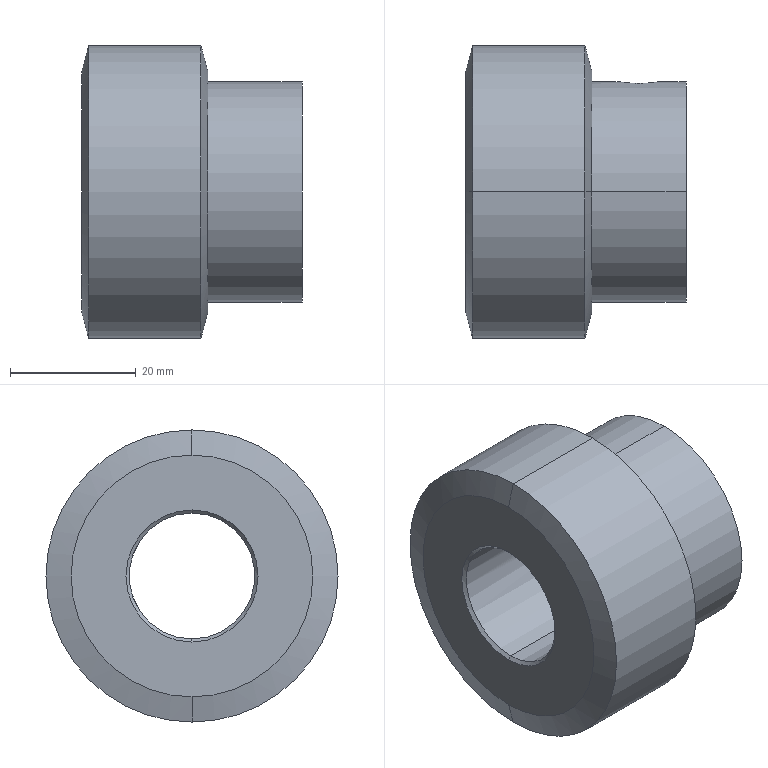Part | SolidWorks | features BaseBody 1 | 1 solid | 26 faces | box 35 x 46.43 x 46.43 mm | volume 36544 mm3 | cone 12 | cylinder 11 | plane 3 | commonest cylinder face diameters 6 x3 4.917 x2 20 x2 35 x2 46.43 x2
STEP:
#1=CARTESIAN_POINT('',(27.5,10.542,-2.459));
#2=VERTEX_POINT('',#1);
#3=CARTESIAN_POINT('',(27.5,10.542,2.459));
#4=VERTEX_POINT('',#3);
#5=CARTESIAN_POINT('',(27.5,10.542,0.));
#6=DIRECTION('',(0.,1.,0.));
#7=DIRECTION('',(0.,0.,1.));
#8=AXIS2_PLACEMENT_3D('',#5,#6,#7);
#9=CIRCLE('',#8,2.459);
#10=EDGE_CURVE('',#2,#4,#9,.T.);
#11=ORIENTED_EDGE('',*,*,#10,.T.);
#12=CARTESIAN_POINT('',(27.5,10.,3.));
#13=VERTEX_POINT('',#12);
#14=CARTESIAN_POINT('',(27.5,10.,3.));
#15=DIRECTION('',(0.,-0.7071,0.7071));
#16=VECTOR('',#15,1000.);
#17=LINE('',#14,#16);
#18=EDGE_CURVE('',#4,#13,#17,.T.);
#19=ORIENTED_EDGE('',*,*,#18,.T.);
#20=CARTESIAN_POINT('',(24.5,10.,0.));
#21=VERTEX_POINT('',#20);
#22=CARTESIAN_POINT('',(27.5,10.,0.));
#23=DIRECTION('',(0.,1.,0.));
#24=DIRECTION('',(0.,0.,1.));
#25=AXIS2_PLACEMENT_3D('',#22,#23,#24);
#26=CIRCLE('',#25,3.);
#27=EDGE_CURVE('',#21,#13,#26,.T.);
#28=ORIENTED_EDGE('',*,*,#27,.F.);
#29=CARTESIAN_POINT('',(27.5,10.,-3.));
#30=VERTEX_POINT('',#29);
#31=CARTESIAN_POINT('',(27.5,10.,0.));
#32=DIRECTION('',(0.,1.,0.));
#33=DIRECTION('',(0.,0.,1.));
#34=AXIS2_PLACEMENT_3D('',#31,#32,#33);
#35=CIRCLE('',#34,3.);
#36=EDGE_CURVE('',#30,#21,#35,.T.);
#37=ORIENTED_EDGE('',*,*,#36,.F.);
#38=CARTESIAN_POINT('',(27.5,10.,-3.));
#39=DIRECTION('',(0.,-0.7071,-0.7071));
#40=VECTOR('',#39,1000.);
#41=LINE('',#38,#40);
#42=EDGE_CURVE('',#2,#30,#41,.T.);
#43=ORIENTED_EDGE('',*,*,#42,.F.);
#44=EDGE_LOOP('',(#11,#19,#28,#37,#43));
#45=FACE_OUTER_BOUND('',#44,.T.);
#46=CARTESIAN_POINT('',(27.5,10.,0.));
#47=DIRECTION('',(0.,-1.,0.));
#48=DIRECTION('',(0.,0.,-1.));
#49=AXIS2_PLACEMENT_3D('',#46,#47,#48);
#50=CONICAL_SURFACE('',#49,3.,0.7854);
#51=ADVANCED_FACE('',(#45),#50,.F.);
#52=ORIENTED_EDGE('',*,*,#10,.F.);
#53=CARTESIAN_POINT('',(27.5,16.959,-2.459));
#54=VERTEX_POINT('',#53);
#55=CARTESIAN_POINT('',(27.5,0.,-2.459));
#56=DIRECTION('',(0.,1.,0.));
#57=VECTOR('',#56,1000.);
#58=LINE('',#55,#57);
#59=EDGE_CURVE('',#2,#54,#58,.T.);
#60=ORIENTED_EDGE('',*,*,#59,.T.);
#61=CARTESIAN_POINT('',(27.5,16.959,2.459));
#62=VERTEX_POINT('',#61);
#63=CARTESIAN_POINT('',(27.5,16.959,0.));
#64=DIRECTION('',(0.,1.,0.));
#65=DIRECTION('',(0.,0.,1.));
#66=AXIS2_PLACEMENT_3D('',#63,#64,#65);
#67=CIRCLE('',#66,2.459);
#68=EDGE_CURVE('',#54,#62,#67,.T.);
#69=ORIENTED_EDGE('',*,*,#68,.T.);
#70=CARTESIAN_POINT('',(27.5,0.,2.459));
#71=DIRECTION('',(0.,1.,0.));
#72=VECTOR('',#71,1000.);
#73=LINE('',#70,#72);
#74=EDGE_CURVE('',#4,#62,#73,.T.);
#75=ORIENTED_EDGE('',*,*,#74,.F.);
#76=EDGE_LOOP('',(#52,#60,#69,#75));
#77=FACE_OUTER_BOUND('',#76,.T.);
#78=CARTESIAN_POINT('',(27.5,0.,0.));
#79=DIRECTION('',(0.,1.,0.));
#80=DIRECTION('',(0.,0.,1.));
#81=AXIS2_PLACEMENT_3D('',#78,#79,#80);
#82=CYLINDRICAL_SURFACE('',#81,2.459);
#83=ADVANCED_FACE('',(#77),#82,.F.);
#84=ORIENTED_EDGE('',*,*,#68,.F.);
#85=CARTESIAN_POINT('',(27.5,17.278,-2.778));
#86=VERTEX_POINT('',#85);
#87=CARTESIAN_POINT('',(27.5,16.959,-2.459));
#88=DIRECTION('',(0.,0.7071,-0.7071));
#89=VECTOR('',#88,1000.);
#90=LINE('',#87,#89);
#91=EDGE_CURVE('',#54,#86,#90,.T.);
#92=ORIENTED_EDGE('',*,*,#91,.T.);
#93=CARTESIAN_POINT('',(27.5,17.278,2.778));
#94=VERTEX_POINT('',#93);
#95=CARTESIAN_POINT('',(27.5,17.278,-2.778));
#96=CARTESIAN_POINT('',(27.309,17.278,-2.778));
#97=CARTESIAN_POINT('',(27.121,17.281,-2.761));
#98=CARTESIAN_POINT('',(26.751,17.291,-2.695));
#99=CARTESIAN_POINT('',(26.567,17.299,-2.646));
#100=CARTESIAN_POINT('',(26.211,17.319,-2.514));
#101=CARTESIAN_POINT('',(26.041,17.33,-2.433));
#102=CARTESIAN_POINT('',(25.718,17.356,-2.24));
#103=CARTESIAN_POINT('',(25.564,17.371,-2.128));
#104=CARTESIAN_POINT('',(25.281,17.4,-1.876));
#105=CARTESIAN_POINT('',(25.154,17.414,-1.739));
#106=CARTESIAN_POINT('',(24.928,17.441,-1.439));
#107=CARTESIAN_POINT('',(24.828,17.454,-1.274));
#108=CARTESIAN_POINT('',(24.668,17.476,-0.9326));
#109=CARTESIAN_POINT('',(24.606,17.485,-0.755));
#110=CARTESIAN_POINT('',(24.522,17.497,-0.3858));
#111=CARTESIAN_POINT('',(24.5,17.5,-0.1944));
#112=CARTESIAN_POINT('',(24.5,17.5,0.1826));
#113=CARTESIAN_POINT('',(24.52,17.497,0.3724));
#114=CARTESIAN_POINT('',(24.603,17.485,0.7441));
#115=CARTESIAN_POINT('',(24.664,17.477,0.9226));
#116=CARTESIAN_POINT('',(24.823,17.455,1.266));
#117=CARTESIAN_POINT('',(24.922,17.442,1.43));
#118=CARTESIAN_POINT('',(25.148,17.415,1.732));
#119=CARTESIAN_POINT('',(25.277,17.4,1.872));
#120=CARTESIAN_POINT('',(25.56,17.371,2.125));
#121=CARTESIAN_POINT('',(25.712,17.357,2.236));
#122=CARTESIAN_POINT('',(26.036,17.331,2.43));
#123=CARTESIAN_POINT('',(26.209,17.319,2.513));
#124=CARTESIAN_POINT('',(26.563,17.299,2.645));
#125=CARTESIAN_POINT('',(26.745,17.291,2.694));
#126=CARTESIAN_POINT('',(27.118,17.281,2.761));
#127=CARTESIAN_POINT('',(27.309,17.278,2.778));
#128=CARTESIAN_POINT('',(27.5,17.278,2.778));
#129=B_SPLINE_CURVE_WITH_KNOTS('',3,(#95,#96,#97,#98,#99,#100,#101,#102,#103,#104,#105,#106,#107,#108,#109,#110,#111,#112,#113,#114,#115,#116,#117,#118,#119,#120,#121,#122,#123,#124,#125,#126,#127,#128),.UNSPECIFIED.,.F.,.F.,(4,2,2,2,2,2,2,2,2,2,2,2,2,2,2,2,4),(0.,0.0005647,0.001129,0.001694,0.002259,0.002823,0.003388,0.003953,0.004517,0.005082,0.005647,0.006211,0.006776,0.007341,0.007905,0.00847,0.009035),.UNSPECIFIED.);
#130=EDGE_CURVE('',#86,#94,#129,.T.);
#131=ORIENTED_EDGE('',*,*,#130,.T.);
#132=CARTESIAN_POINT('',(27.5,16.959,2.459));
#133=DIRECTION('',(0.,0.7071,0.7071));
#134=VECTOR('',#133,1000.);
#135=LINE('',#132,#134);
#136=EDGE_CURVE('',#62,#94,#135,.T.);
#137=ORIENTED_EDGE('',*,*,#136,.F.);
#138=EDGE_LOOP('',(#84,#92,#131,#137));
#139=FACE_OUTER_BOUND('',#138,.T.);
#140=CARTESIAN_POINT('',(27.5,16.959,0.));
#141=DIRECTION('',(0.,1.,0.));
#142=DIRECTION('',(0.,0.,1.));
#143=AXIS2_PLACEMENT_3D('',#140,#141,#142);
#144=CONICAL_SURFACE('',#143,2.459,0.7854);
#145=ADVANCED_FACE('',(#139),#144,.F.);
#146=CARTESIAN_POINT('',(30.5,10.,0.));
#147=VERTEX_POINT('',#146);
#148=CARTESIAN_POINT('',(27.5,9.539,3.));
#149=VERTEX_POINT('',#148);
#150=CARTESIAN_POINT('',(30.5,10.,0.));
#151=CARTESIAN_POINT('',(30.5,10.,0.1993));
#152=CARTESIAN_POINT('',(30.48,9.994,0.3951));
#153=CARTESIAN_POINT('',(30.403,9.971,0.7799));
#154=CARTESIAN_POINT('',(30.345,9.954,0.971));
#155=CARTESIAN_POINT('',(30.194,9.912,1.334));
#156=CARTESIAN_POINT('',(30.102,9.887,1.505));
#157=CARTESIAN_POINT('',(29.885,9.832,1.831));
#158=CARTESIAN_POINT('',(29.759,9.802,1.984));
#159=CARTESIAN_POINT('',(29.347,9.713,2.396));
#160=CARTESIAN_POINT('',(29.014,9.652,2.619));
#161=CARTESIAN_POINT('',(28.474,9.587,2.844));
#162=CARTESIAN_POINT('',(28.284,9.57,2.902));
#163=CARTESIAN_POINT('',(27.896,9.546,2.98));
#164=CARTESIAN_POINT('',(27.699,9.539,3.));
#165=CARTESIAN_POINT('',(27.5,9.539,3.));
#166=B_SPLINE_CURVE_WITH_KNOTS('',3,(#150,#151,#152,#153,#154,#155,#156,#157,#158,#159,#160,#161,#162,#163,#164,#165),.UNSPECIFIED.,.F.,.F.,(4,2,2,2,2,2,2,4),(0.,0.0005892,0.001178,0.001768,0.002357,0.003535,0.004125,0.004714),.UNSPECIFIED.);
#167=EDGE_CURVE('',#147,#149,#166,.T.);
#168=ORIENTED_EDGE('',*,*,#167,.T.);
#169=CARTESIAN_POINT('',(27.5,0.,3.));
#170=DIRECTION('',(0.,1.,0.));
#171=VECTOR('',#170,1000.);
#172=LINE('',#169,#171);
#173=EDGE_CURVE('',#149,#13,#172,.T.);
#174=ORIENTED_EDGE('',*,*,#173,.T.);
#175=CARTESIAN_POINT('',(27.5,10.,0.));
#176=DIRECTION('',(0.,1.,0.));
#177=DIRECTION('',(0.,0.,1.));
#178=AXIS2_PLACEMENT_3D('',#175,#176,#177);
#179=CIRCLE('',#178,3.);
#180=EDGE_CURVE('',#13,#147,#179,.T.);
#181=ORIENTED_EDGE('',*,*,#180,.T.);
#182=EDGE_LOOP('',(#168,#174,#181));
#183=FACE_OUTER_BOUND('',#182,.T.);
#184=CARTESIAN_POINT('',(27.5,0.,0.));
#185=DIRECTION('',(0.,1.,0.));
#186=DIRECTION('',(0.,0.,1.));
#187=AXIS2_PLACEMENT_3D('',#184,#185,#186);
#188=CYLINDRICAL_SURFACE('',#187,3.);
#189=ADVANCED_FACE('',(#183),#188,.F.);
#190=CARTESIAN_POINT('',(18.928,0.,23.215));
#191=VERTEX_POINT('',#190);
#192=CARTESIAN_POINT('',(18.928,0.,-23.215));
#193=VERTEX_POINT('',#192);
#194=CARTESIAN_POINT('',(18.928,0.,0.));
#195=DIRECTION('',(-1.,0.,0.));
#196=DIRECTION('',(0.,0.,1.));
#197=AXIS2_PLACEMENT_3D('',#194,#195,#196);
#198=CIRCLE('',#197,23.215);
#199=EDGE_CURVE('',#191,#193,#198,.T.);
#200=ORIENTED_EDGE('',*,*,#199,.T.);
#201=CARTESIAN_POINT('',(1.072,0.,-23.215));
#202=VERTEX_POINT('',#201);
#203=CARTESIAN_POINT('',(35.,0.,-23.215));
#204=DIRECTION('',(-1.,0.,0.));
#205=VECTOR('',#204,1000.);
#206=LINE('',#203,#205);
#207=EDGE_CURVE('',#193,#202,#206,.T.);
#208=ORIENTED_EDGE('',*,*,#207,.T.);
#209=CARTESIAN_POINT('',(1.072,0.,23.215));
#210=VERTEX_POINT('',#209);
#211=CARTESIAN_POINT('',(1.072,0.,0.));
#212=DIRECTION('',(-1.,0.,0.));
#213=DIRECTION('',(0.,0.,1.));
#214=AXIS2_PLACEMENT_3D('',#211,#212,#213);
#215=CIRCLE('',#214,23.215);
#216=EDGE_CURVE('',#210,#202,#215,.T.);
#217=ORIENTED_EDGE('',*,*,#216,.F.);
#218=CARTESIAN_POINT('',(35.,0.,23.215));
#219=DIRECTION('',(-1.,0.,0.));
#220=VECTOR('',#219,1000.);
#221=LINE('',#218,#220);
#222=EDGE_CURVE('',#191,#210,#221,.T.);
#223=ORIENTED_EDGE('',*,*,#222,.F.);
#224=EDGE_LOOP('',(#200,#208,#217,#223));
#225=FACE_OUTER_BOUND('',#224,.T.);
#226=CARTESIAN_POINT('',(35.,0.,0.));
#227=DIRECTION('',(-1.,0.,0.));
#228=DIRECTION('',(0.,0.,1.));
#229=AXIS2_PLACEMENT_3D('',#226,#227,#228);
#230=CYLINDRICAL_SURFACE('',#229,23.215);
#231=ADVANCED_FACE('',(#225),#230,.T.);
#232=CARTESIAN_POINT('',(20.,0.,19.215));
#233=VERTEX_POINT('',#232);
#234=CARTESIAN_POINT('',(20.,0.,-19.215));
#235=VERTEX_POINT('',#234);
#236=CARTESIAN_POINT('',(20.,0.,0.));
#237=DIRECTION('',(-1.,0.,0.));
#238=DIRECTION('',(0.,0.,1.));
#239=AXIS2_PLACEMENT_3D('',#236,#237,#238);
#240=CIRCLE('',#239,19.215);
#241=EDGE_CURVE('',#233,#235,#240,.T.);
#242=ORIENTED_EDGE('',*,*,#241,.T.);
#243=CARTESIAN_POINT('',(20.,0.,-19.215));
#244=DIRECTION('',(-0.2588,0.,-0.9659));
#245=VECTOR('',#244,1000.);
#246=LINE('',#243,#245);
#247=EDGE_CURVE('',#235,#193,#246,.T.);
#248=ORIENTED_EDGE('',*,*,#247,.T.);
#249=ORIENTED_EDGE('',*,*,#199,.F.);
#250=CARTESIAN_POINT('',(20.,0.,19.215));
#251=DIRECTION('',(-0.2588,0.,0.9659));
#252=VECTOR('',#251,1000.);
#253=LINE('',#250,#252);
#254=EDGE_CURVE('',#233,#191,#253,.T.);
#255=ORIENTED_EDGE('',*,*,#254,.F.);
#256=EDGE_LOOP('',(#242,#248,#249,#255));
#257=FACE_OUTER_BOUND('',#256,.T.);
#258=CARTESIAN_POINT('',(20.,0.,0.));
#259=DIRECTION('',(-1.,0.,0.));
#260=DIRECTION('',(0.,0.,1.));
#261=AXIS2_PLACEMENT_3D('',#258,#259,#260);
#262=CONICAL_SURFACE('',#261,19.215,1.309);
#263=ADVANCED_FACE('',(#257),#262,.T.);
#264=CARTESIAN_POINT('',(34.5,0.,-10.));
#265=VERTEX_POINT('',#264);
#266=CARTESIAN_POINT('',(34.5,0.,10.));
#267=VERTEX_POINT('',#266);
#268=CARTESIAN_POINT('',(34.5,0.,0.));
#269=DIRECTION('',(-1.,0.,0.));
#270=DIRECTION('',(0.,0.,1.));
#271=AXIS2_PLACEMENT_3D('',#268,#269,#270);
#272=CIRCLE('',#271,10.);
#273=EDGE_CURVE('',#265,#267,#272,.T.);
#274=ORIENTED_EDGE('',*,*,#273,.T.);
#275=CARTESIAN_POINT('',(35.,0.,10.5));
#276=VERTEX_POINT('',#275);
#277=CARTESIAN_POINT('',(34.5,0.,10.));
#278=DIRECTION('',(0.7071,0.,0.7071));
#279=VECTOR('',#278,1000.);
#280=LINE('',#277,#279);
#281=EDGE_CURVE('',#267,#276,#280,.T.);
#282=ORIENTED_EDGE('',*,*,#281,.T.);
#283=CARTESIAN_POINT('',(35.,0.,-10.5));
#284=VERTEX_POINT('',#283);
#285=CARTESIAN_POINT('',(35.,0.,0.));
#286=DIRECTION('',(-1.,0.,0.));
#287=DIRECTION('',(0.,0.,1.));
#288=AXIS2_PLACEMENT_3D('',#285,#286,#287);
#289=CIRCLE('',#288,10.5);
#290=EDGE_CURVE('',#284,#276,#289,.T.);
#291=ORIENTED_EDGE('',*,*,#290,.F.);
#292=CARTESIAN_POINT('',(34.5,0.,-10.));
#293=DIRECTION('',(0.7071,0.,-0.7071));
#294=VECTOR('',#293,1000.);
#295=LINE('',#292,#294);
#296=EDGE_CURVE('',#265,#284,#295,.T.);
#297=ORIENTED_EDGE('',*,*,#296,.F.);
#298=EDGE_LOOP('',(#274,#282,#291,#297));
#299=FACE_OUTER_BOUND('',#298,.T.);
#300=CARTESIAN_POINT('',(34.5,0.,0.));
#301=DIRECTION('',(1.,0.,0.));
#302=DIRECTION('',(0.,0.,-1.));
#303=AXIS2_PLACEMENT_3D('',#300,#301,#302);
#304=CONICAL_SURFACE('',#303,10.,0.7854);
#305=ADVANCED_FACE('',(#299),#304,.F.);
#306=CARTESIAN_POINT('',(0.5,0.,-10.));
#307=VERTEX_POINT('',#306);
#308=CARTESIAN_POINT('',(0.5,0.,10.));
#309=VERTEX_POINT('',#308);
#310=CARTESIAN_POINT('',(0.5,0.,0.));
#311=DIRECTION('',(-1.,0.,0.));
#312=DIRECTION('',(0.,0.,1.));
#313=AXIS2_PLACEMENT_3D('',#310,#311,#312);
#314=CIRCLE('',#313,10.);
#315=EDGE_CURVE('',#307,#309,#314,.T.);
#316=ORIENTED_EDGE('',*,*,#315,.F.);
#317=CARTESIAN_POINT('',(0.,0.,-10.5));
#318=VERTEX_POINT('',#317);
#319=CARTESIAN_POINT('',(0.,0.,-10.5));
#320=DIRECTION('',(-0.7071,0.,-0.7071));
#321=VECTOR('',#320,1000.);
#322=LINE('',#319,#321);
#323=EDGE_CURVE('',#307,#318,#322,.T.);
#324=ORIENTED_EDGE('',*,*,#323,.T.);
#325=CARTESIAN_POINT('',(0.,0.,10.5));
#326=VERTEX_POINT('',#325);
#327=CARTESIAN_POINT('',(0.,0.,0.));
#328=DIRECTION('',(-1.,0.,0.));
#329=DIRECTION('',(0.,0.,1.));
#330=AXIS2_PLACEMENT_3D('',#327,#328,#329);
#331=CIRCLE('',#330,10.5);
#332=EDGE_CURVE('',#318,#326,#331,.T.);
#333=ORIENTED_EDGE('',*,*,#332,.T.);
#334=CARTESIAN_POINT('',(0.,0.,10.5));
#335=DIRECTION('',(-0.7071,0.,0.7071));
#336=VECTOR('',#335,1000.);
#337=LINE('',#334,#336);
#338=EDGE_CURVE('',#309,#326,#337,.T.);
#339=ORIENTED_EDGE('',*,*,#338,.F.);
#340=EDGE_LOOP('',(#316,#324,#333,#339));
#341=FACE_OUTER_BOUND('',#340,.T.);
#342=CARTESIAN_POINT('',(0.,0.,0.));
#343=DIRECTION('',(-1.,0.,0.));
#344=DIRECTION('',(0.,0.,1.));
#345=AXIS2_PLACEMENT_3D('',#342,#343,#344);
#346=CONICAL_SURFACE('',#345,10.5,0.7854);
#347=ADVANCED_FACE('',(#341),#346,.F.);
#348=CARTESIAN_POINT('',(0.,0.,19.215));
#349=VERTEX_POINT('',#348);
#350=CARTESIAN_POINT('',(0.,0.,-19.215));
#351=VERTEX_POINT('',#350);
#352=CARTESIAN_POINT('',(0.,0.,0.));
#353=DIRECTION('',(-1.,0.,0.));
#354=DIRECTION('',(0.,0.,1.));
#355=AXIS2_PLACEMENT_3D('',#352,#353,#354);
#356=CIRCLE('',#355,19.215);
#357=EDGE_CURVE('',#349,#351,#356,.T.);
#358=ORIENTED_EDGE('',*,*,#357,.F.);
#359=CARTESIAN_POINT('',(1.072,0.,23.215));
#360=DIRECTION('',(0.2588,0.,0.9659));
#361=VECTOR('',#360,1000.);
#362=LINE('',#359,#361);
#363=EDGE_CURVE('',#349,#210,#362,.T.);
#364=ORIENTED_EDGE('',*,*,#363,.T.);
#365=ORIENTED_EDGE('',*,*,#216,.T.);
#366=CARTESIAN_POINT('',(1.072,0.,-23.215));
#367=DIRECTION('',(0.2588,0.,-0.9659));
#368=VECTOR('',#367,1000.);
#369=LINE('',#366,#368);
#370=EDGE_CURVE('',#351,#202,#369,.T.);
#371=ORIENTED_EDGE('',*,*,#370,.F.);
#372=EDGE_LOOP('',(#358,#364,#365,#371));
#373=FACE_OUTER_BOUND('',#372,.T.);
#374=CARTESIAN_POINT('',(1.072,0.,0.));
#375=DIRECTION('',(1.,0.,0.));
#376=DIRECTION('',(0.,0.,-1.));
#377=AXIS2_PLACEMENT_3D('',#374,#375,#376);
#378=CONICAL_SURFACE('',#377,23.215,1.309);
#379=ADVANCED_FACE('',(#373),#378,.T.);
#380=CARTESIAN_POINT('',(27.5,17.278,2.778));
#381=CARTESIAN_POINT('',(27.691,17.278,2.778));
#382=CARTESIAN_POINT('',(27.879,17.281,2.761));
#383=CARTESIAN_POINT('',(28.249,17.291,2.695));
#384=CARTESIAN_POINT('',(28.433,17.299,2.646));
#385=CARTESIAN_POINT('',(28.789,17.319,2.514));
#386=CARTESIAN_POINT('',(28.959,17.33,2.433));
#387=CARTESIAN_POINT('',(29.282,17.356,2.24));
#388=CARTESIAN_POINT('',(29.436,17.371,2.128));
#389=CARTESIAN_POINT('',(29.719,17.4,1.876));
#390=CARTESIAN_POINT('',(29.846,17.414,1.739));
#391=CARTESIAN_POINT('',(30.072,17.441,1.439));
#392=CARTESIAN_POINT('',(30.172,17.454,1.274));
#393=CARTESIAN_POINT('',(30.332,17.476,0.9326));
#394=CARTESIAN_POINT('',(30.394,17.485,0.755));
#395=CARTESIAN_POINT('',(30.478,17.497,0.3858));
#396=CARTESIAN_POINT('',(30.5,17.5,0.1944));
#397=CARTESIAN_POINT('',(30.5,17.5,-0.1826));
#398=CARTESIAN_POINT('',(30.48,17.497,-0.3724));
#399=CARTESIAN_POINT('',(30.397,17.485,-0.7441));
#400=CARTESIAN_POINT('',(30.336,17.477,-0.9226));
#401=CARTESIAN_POINT('',(30.177,17.455,-1.266));
#402=CARTESIAN_POINT('',(30.078,17.442,-1.43));
#403=CARTESIAN_POINT('',(29.852,17.415,-1.732));
#404=CARTESIAN_POINT('',(29.723,17.4,-1.872));
#405=CARTESIAN_POINT('',(29.44,17.371,-2.125));
#406=CARTESIAN_POINT('',(29.288,17.357,-2.236));
#407=CARTESIAN_POINT('',(28.964,17.331,-2.43));
#408=CARTESIAN_POINT('',(28.791,17.319,-2.513));
#409=CARTESIAN_POINT('',(28.437,17.299,-2.645));
#410=CARTESIAN_POINT('',(28.255,17.291,-2.694));
#411=CARTESIAN_POINT('',(27.882,17.281,-2.761));
#412=CARTESIAN_POINT('',(27.691,17.278,-2.778));
#413=CARTESIAN_POINT('',(27.5,17.278,-2.778));
#414=B_SPLINE_CURVE_WITH_KNOTS('',3,(#380,#381,#382,#383,#384,#385,#386,#387,#388,#389,#390,#391,#392,#393,#394,#395,#396,#397,#398,#399,#400,#401,#402,#403,#404,#405,#406,#407,#408,#409,#410,#411,#412,#413),.UNSPECIFIED.,.F.,.F.,(4,2,2,2,2,2,2,2,2,2,2,2,2,2,2,2,4),(0.009035,0.009599,0.01016,0.01073,0.01129,0.01186,0.01242,0.01299,0.01355,0.01411,0.01468,0.01524,0.01581,0.01637,0.01694,0.0175,0.01806),.UNSPECIFIED.);
#415=EDGE_CURVE('',#94,#86,#414,.T.);
#416=ORIENTED_EDGE('',*,*,#415,.F.);
#417=ORIENTED_EDGE('',*,*,#130,.F.);
#418=EDGE_LOOP('',(#416,#417));
#419=FACE_BOUND('',#418,.T.);
#420=CARTESIAN_POINT('',(35.,0.,17.5));
#421=VERTEX_POINT('',#420);
#422=CARTESIAN_POINT('',(35.,0.,-17.5));
#423=VERTEX_POINT('',#422);
#424=CARTESIAN_POINT('',(35.,0.,0.));
#425=DIRECTION('',(-1.,0.,0.));
#426=DIRECTION('',(0.,0.,1.));
#427=AXIS2_PLACEMENT_3D('',#424,#425,#426);
#428=CIRCLE('',#427,17.5);
#429=EDGE_CURVE('',#421,#423,#428,.T.);
#430=ORIENTED_EDGE('',*,*,#429,.T.);
#431=CARTESIAN_POINT('',(20.,0.,-17.5));
#432=VERTEX_POINT('',#431);
#433=CARTESIAN_POINT('',(35.,0.,-17.5));
#434=DIRECTION('',(-1.,0.,0.));
#435=VECTOR('',#434,1000.);
#436=LINE('',#433,#435);
#437=EDGE_CURVE('',#423,#432,#436,.T.);
#438=ORIENTED_EDGE('',*,*,#437,.T.);
#439=CARTESIAN_POINT('',(20.,0.,17.5));
#440=VERTEX_POINT('',#439);
#441=CARTESIAN_POINT('',(20.,0.,0.));
#442=DIRECTION('',(-1.,0.,0.));
#443=DIRECTION('',(0.,0.,1.));
#444=AXIS2_PLACEMENT_3D('',#441,#442,#443);
#445=CIRCLE('',#444,17.5);
#446=EDGE_CURVE('',#440,#432,#445,.T.);
#447=ORIENTED_EDGE('',*,*,#446,.F.);
#448=CARTESIAN_POINT('',(35.,0.,17.5));
#449=DIRECTION('',(-1.,0.,0.));
#450=VECTOR('',#449,1000.);
#451=LINE('',#448,#450);
#452=EDGE_CURVE('',#421,#440,#451,.T.);
#453=ORIENTED_EDGE('',*,*,#452,.F.);
#454=EDGE_LOOP('',(#430,#438,#447,#453));
#455=FACE_OUTER_BOUND('',#454,.T.);
#456=CARTESIAN_POINT('',(35.,0.,0.));
#457=DIRECTION('',(-1.,0.,0.));
#458=DIRECTION('',(0.,0.,1.));
#459=AXIS2_PLACEMENT_3D('',#456,#457,#458);
#460=CYLINDRICAL_SURFACE('',#459,17.5);
#461=ADVANCED_FACE('',(#419,#455),#460,.T.);
#462=ORIENTED_EDGE('',*,*,#273,.F.);
#463=CARTESIAN_POINT('',(35.,0.,-10.));
#464=DIRECTION('',(-1.,0.,0.));
#465=VECTOR('',#464,1000.);
#466=LINE('',#463,#465);
#467=EDGE_CURVE('',#265,#307,#466,.T.);
#468=ORIENTED_EDGE('',*,*,#467,.T.);
#469=ORIENTED_EDGE('',*,*,#315,.T.);
#470=CARTESIAN_POINT('',(35.,0.,10.));
#471=DIRECTION('',(-1.,0.,0.));
#472=VECTOR('',#471,1000.);
#473=LINE('',#470,#472);
#474=EDGE_CURVE('',#267,#309,#473,.T.);
#475=ORIENTED_EDGE('',*,*,#474,.F.);
#476=EDGE_LOOP('',(#462,#468,#469,#475));
#477=FACE_OUTER_BOUND('',#476,.T.);
#478=CARTESIAN_POINT('',(35.,0.,0.));
#479=DIRECTION('',(-1.,0.,0.));
#480=DIRECTION('',(0.,0.,1.));
#481=AXIS2_PLACEMENT_3D('',#478,#479,#480);
#482=CYLINDRICAL_SURFACE('',#481,10.);
#483=ADVANCED_FACE('',(#477),#482,.F.);
#484=CARTESIAN_POINT('',(24.5,10.,0.));
#485=CARTESIAN_POINT('',(24.5,10.,-0.1994));
#486=CARTESIAN_POINT('',(24.52,9.994,-0.3952));
#487=CARTESIAN_POINT('',(24.597,9.971,-0.7801));
#488=CARTESIAN_POINT('',(24.655,9.954,-0.9713));
#489=CARTESIAN_POINT('',(24.806,9.912,-1.334));
#490=CARTESIAN_POINT('',(24.898,9.887,-1.506));
#491=CARTESIAN_POINT('',(25.116,9.832,-1.831));
#492=CARTESIAN_POINT('',(25.241,9.802,-1.984));
#493=CARTESIAN_POINT('',(25.654,9.713,-2.396));
#494=CARTESIAN_POINT('',(25.986,9.652,-2.619));
#495=CARTESIAN_POINT('',(26.527,9.587,-2.844));
#496=CARTESIAN_POINT('',(26.717,9.57,-2.903));
#497=CARTESIAN_POINT('',(27.105,9.546,-2.98));
#498=CARTESIAN_POINT('',(27.3,9.539,-3.));
#499=CARTESIAN_POINT('',(27.694,9.539,-3.));
#500=CARTESIAN_POINT('',(27.894,9.546,-2.981));
#501=CARTESIAN_POINT('',(28.28,9.569,-2.904));
#502=CARTESIAN_POINT('',(28.467,9.587,-2.847));
#503=CARTESIAN_POINT('',(28.832,9.63,-2.695));
#504=CARTESIAN_POINT('',(29.005,9.656,-2.602));
#505=CARTESIAN_POINT('',(29.329,9.712,-2.386));
#506=CARTESIAN_POINT('',(29.482,9.742,-2.261));
#507=CARTESIAN_POINT('',(29.759,9.802,-1.984));
#508=CARTESIAN_POINT('',(29.882,9.832,-1.834));
#509=CARTESIAN_POINT('',(30.1,9.887,-1.51));
#510=CARTESIAN_POINT('',(30.194,9.912,-1.334));
#511=CARTESIAN_POINT('',(30.345,9.954,-0.9731));
#512=CARTESIAN_POINT('',(30.402,9.971,-0.786));
#513=CARTESIAN_POINT('',(30.48,9.994,-0.3988));
#514=CARTESIAN_POINT('',(30.5,10.,-0.1994));
#515=CARTESIAN_POINT('',(30.5,10.,0.));
#516=B_SPLINE_CURVE_WITH_KNOTS('',3,(#484,#485,#486,#487,#488,#489,#490,#491,#492,#493,#494,#495,#496,#497,#498,#499,#500,#501,#502,#503,#504,#505,#506,#507,#508,#509,#510,#511,#512,#513,#514,#515),.UNSPECIFIED.,.F.,.F.,(4,2,2,2,2,2,2,2,2,2,2,2,2,2,2,4),(0.,0.0005894,0.001179,0.001768,0.002358,0.003537,0.004126,0.004715,0.005305,0.005894,0.006484,0.007073,0.007662,0.008252,0.008841,0.009431),.UNSPECIFIED.);
#517=EDGE_CURVE('',#21,#147,#516,.T.);
#518=ORIENTED_EDGE('',*,*,#517,.T.);
#519=CARTESIAN_POINT('',(27.5,10.,0.));
#520=DIRECTION('',(0.,1.,0.));
#521=DIRECTION('',(0.,0.,1.));
#522=AXIS2_PLACEMENT_3D('',#519,#520,#521);
#523=CIRCLE('',#522,3.);
#524=EDGE_CURVE('',#147,#30,#523,.T.);
#525=ORIENTED_EDGE('',*,*,#524,.T.);
#526=ORIENTED_EDGE('',*,*,#36,.T.);
#527=EDGE_LOOP('',(#518,#525,#526));
#528=FACE_OUTER_BOUND('',#527,.T.);
#529=CARTESIAN_POINT('',(27.5,0.,0.));
#530=DIRECTION('',(0.,1.,0.));
#531=DIRECTION('',(0.,0.,1.));
#532=AXIS2_PLACEMENT_3D('',#529,#530,#531);
#533=CYLINDRICAL_SURFACE('',#532,3.);
#534=ADVANCED_FACE('',(#528),#533,.F.);
#535=ORIENTED_EDGE('',*,*,#446,.T.);
#536=CARTESIAN_POINT('',(20.,0.,0.));
#537=DIRECTION('',(-1.,0.,0.));
#538=DIRECTION('',(0.,0.,1.));
#539=AXIS2_PLACEMENT_3D('',#536,#537,#538);
#540=CIRCLE('',#539,17.5);
#541=EDGE_CURVE('',#432,#440,#540,.T.);
#542=ORIENTED_EDGE('',*,*,#541,.T.);
#543=EDGE_LOOP('',(#535,#542));
#544=FACE_BOUND('',#543,.T.);
#545=ORIENTED_EDGE('',*,*,#241,.F.);
#546=CARTESIAN_POINT('',(20.,0.,0.));
#547=DIRECTION('',(-1.,0.,0.));
#548=DIRECTION('',(0.,0.,1.));
#549=AXIS2_PLACEMENT_3D('',#546,#547,#548);
#550=CIRCLE('',#549,19.215);
#551=EDGE_CURVE('',#235,#233,#550,.T.);
#552=ORIENTED_EDGE('',*,*,#551,.F.);
#553=EDGE_LOOP('',(#545,#552));
#554=FACE_OUTER_BOUND('',#553,.T.);
#555=CARTESIAN_POINT('',(20.,17.5,0.));
#556=DIRECTION('',(-1.,0.,0.));
#557=DIRECTION('',(0.,0.,1.));
#558=AXIS2_PLACEMENT_3D('',#555,#556,#557);
#559=PLANE('',#558);
#560=ADVANCED_FACE('',(#544,#554),#559,.F.);
#561=ORIENTED_EDGE('',*,*,#290,.T.);
#562=CARTESIAN_POINT('',(35.,0.,0.));
#563=DIRECTION('',(-1.,0.,0.));
#564=DIRECTION('',(0.,0.,1.));
#565=AXIS2_PLACEMENT_3D('',#562,#563,#564);
#566=CIRCLE('',#565,10.5);
#567=EDGE_CURVE('',#276,#284,#566,.T.);
#568=ORIENTED_EDGE('',*,*,#567,.T.);
#569=EDGE_LOOP('',(#561,#568));
#570=FACE_BOUND('',#569,.T.);
#571=ORIENTED_EDGE('',*,*,#429,.F.);
#572=CARTESIAN_POINT('',(35.,0.,0.));
#573=DIRECTION('',(-1.,0.,0.));
#574=DIRECTION('',(0.,0.,1.));
#575=AXIS2_PLACEMENT_3D('',#572,#573,#574);
#576=CIRCLE('',#575,17.5);
#577=EDGE_CURVE('',#423,#421,#576,.T.);
#578=ORIENTED_EDGE('',*,*,#577,.F.);
#579=EDGE_LOOP('',(#571,#578));
#580=FACE_OUTER_BOUND('',#579,.T.);
#581=CARTESIAN_POINT('',(35.,10.5,0.));
#582=DIRECTION('',(-1.,0.,0.));
#583=DIRECTION('',(0.,0.,1.));
#584=AXIS2_PLACEMENT_3D('',#581,#582,#583);
#585=PLANE('',#584);
#586=ADVANCED_FACE('',(#570,#580),#585,.F.);
#587=CARTESIAN_POINT('',(0.,0.,0.));
#588=DIRECTION('',(-1.,0.,0.));
#589=DIRECTION('',(0.,0.,1.));
#590=AXIS2_PLACEMENT_3D('',#587,#588,#589);
#591=CIRCLE('',#590,10.5);
#592=EDGE_CURVE('',#326,#318,#591,.T.);
#593=ORIENTED_EDGE('',*,*,#592,.F.);
#594=ORIENTED_EDGE('',*,*,#332,.F.);
#595=EDGE_LOOP('',(#593,#594));
#596=FACE_BOUND('',#595,.T.);
#597=CARTESIAN_POINT('',(0.,0.,0.));
#598=DIRECTION('',(-1.,0.,0.));
#599=DIRECTION('',(0.,0.,1.));
#600=AXIS2_PLACEMENT_3D('',#597,#598,#599);
#601=CIRCLE('',#600,19.215);
#602=EDGE_CURVE('',#351,#349,#601,.T.);
#603=ORIENTED_EDGE('',*,*,#602,.T.);
#604=ORIENTED_EDGE('',*,*,#357,.T.);
#605=EDGE_LOOP('',(#603,#604));
#606=FACE_OUTER_BOUND('',#605,.T.);
#607=CARTESIAN_POINT('',(0.,19.215,0.));
#608=DIRECTION('',(1.,0.,0.));
#609=DIRECTION('',(0.,1.,0.));
#610=AXIS2_PLACEMENT_3D('',#607,#608,#609);
#611=PLANE('',#610);
#612=ADVANCED_FACE('',(#596,#606),#611,.F.);
#613=ORIENTED_EDGE('',*,*,#467,.F.);
#614=CARTESIAN_POINT('',(34.5,0.,0.));
#615=DIRECTION('',(-1.,0.,0.));
#616=DIRECTION('',(0.,0.,1.));
#617=AXIS2_PLACEMENT_3D('',#614,#615,#616);
#618=CIRCLE('',#617,10.);
#619=EDGE_CURVE('',#267,#265,#618,.T.);
#620=ORIENTED_EDGE('',*,*,#619,.F.);
#621=ORIENTED_EDGE('',*,*,#474,.T.);
#622=CARTESIAN_POINT('',(0.5,0.,0.));
#623=DIRECTION('',(-1.,0.,0.));
#624=DIRECTION('',(0.,0.,1.));
#625=AXIS2_PLACEMENT_3D('',#622,#623,#624);
#626=CIRCLE('',#625,10.);
#627=EDGE_CURVE('',#309,#307,#626,.T.);
#628=ORIENTED_EDGE('',*,*,#627,.T.);
#629=EDGE_LOOP('',(#613,#620,#621,#628));
#630=FACE_OUTER_BOUND('',#629,.T.);
#631=ORIENTED_EDGE('',*,*,#517,.F.);
#632=CARTESIAN_POINT('',(27.5,9.539,3.));
#633=CARTESIAN_POINT('',(27.301,9.539,3.));
#634=CARTESIAN_POINT('',(27.105,9.546,2.98));
#635=CARTESIAN_POINT('',(26.72,9.569,2.904));
#636=CARTESIAN_POINT('',(26.529,9.587,2.845));
#637=CARTESIAN_POINT('',(26.167,9.63,2.695));
#638=CARTESIAN_POINT('',(25.995,9.656,2.602));
#639=CARTESIAN_POINT('',(25.67,9.712,2.385));
#640=CARTESIAN_POINT('',(25.517,9.742,2.259));
#641=CARTESIAN_POINT('',(25.104,9.832,1.847));
#642=CARTESIAN_POINT('',(24.881,9.891,1.515));
#643=CARTESIAN_POINT('',(24.656,9.954,0.9743));
#644=CARTESIAN_POINT('',(24.598,9.971,0.7845));
#645=CARTESIAN_POINT('',(24.52,9.994,0.3961));
#646=CARTESIAN_POINT('',(24.5,10.,0.1993));
#647=CARTESIAN_POINT('',(24.5,10.,0.));
#648=B_SPLINE_CURVE_WITH_KNOTS('',3,(#632,#633,#634,#635,#636,#637,#638,#639,#640,#641,#642,#643,#644,#645,#646,#647),.UNSPECIFIED.,.F.,.F.,(4,2,2,2,2,2,2,4),(0.004714,0.005303,0.005892,0.006482,0.007071,0.008249,0.008839,0.009428),.UNSPECIFIED.);
#649=EDGE_CURVE('',#149,#21,#648,.T.);
#650=ORIENTED_EDGE('',*,*,#649,.F.);
#651=ORIENTED_EDGE('',*,*,#167,.F.);
#652=EDGE_LOOP('',(#631,#650,#651));
#653=FACE_BOUND('',#652,.T.);
#654=CARTESIAN_POINT('',(35.,0.,0.));
#655=DIRECTION('',(-1.,0.,0.));
#656=DIRECTION('',(0.,0.,1.));
#657=AXIS2_PLACEMENT_3D('',#654,#655,#656);
#658=CYLINDRICAL_SURFACE('',#657,10.);
#659=ADVANCED_FACE('',(#630,#653),#658,.F.);
#660=ORIENTED_EDGE('',*,*,#437,.F.);
#661=ORIENTED_EDGE('',*,*,#577,.T.);
#662=ORIENTED_EDGE('',*,*,#452,.T.);
#663=ORIENTED_EDGE('',*,*,#541,.F.);
#664=EDGE_LOOP('',(#660,#661,#662,#663));
#665=FACE_OUTER_BOUND('',#664,.T.);
#666=CARTESIAN_POINT('',(35.,0.,0.));
#667=DIRECTION('',(-1.,0.,0.));
#668=DIRECTION('',(0.,0.,1.));
#669=AXIS2_PLACEMENT_3D('',#666,#667,#668);
#670=CYLINDRICAL_SURFACE('',#669,17.5);
#671=ADVANCED_FACE('',(#665),#670,.T.);
#672=ORIENTED_EDGE('',*,*,#363,.F.);
#673=ORIENTED_EDGE('',*,*,#602,.F.);
#674=ORIENTED_EDGE('',*,*,#370,.T.);
#675=CARTESIAN_POINT('',(1.072,0.,0.));
#676=DIRECTION('',(-1.,0.,0.));
#677=DIRECTION('',(0.,0.,1.));
#678=AXIS2_PLACEMENT_3D('',#675,#676,#677);
#679=CIRCLE('',#678,23.215);
#680=EDGE_CURVE('',#202,#210,#679,.T.);
#681=ORIENTED_EDGE('',*,*,#680,.T.);
#682=EDGE_LOOP('',(#672,#673,#674,#681));
#683=FACE_OUTER_BOUND('',#682,.T.);
#684=CARTESIAN_POINT('',(1.072,0.,0.));
#685=DIRECTION('',(1.,0.,0.));
#686=DIRECTION('',(0.,0.,-1.));
#687=AXIS2_PLACEMENT_3D('',#684,#685,#686);
#688=CONICAL_SURFACE('',#687,23.215,1.309);
#689=ADVANCED_FACE('',(#683),#688,.T.);
#690=ORIENTED_EDGE('',*,*,#323,.F.);
#691=ORIENTED_EDGE('',*,*,#627,.F.);
#692=ORIENTED_EDGE('',*,*,#338,.T.);
#693=ORIENTED_EDGE('',*,*,#592,.T.);
#694=EDGE_LOOP('',(#690,#691,#692,#693));
#695=FACE_OUTER_BOUND('',#694,.T.);
#696=CARTESIAN_POINT('',(0.,0.,0.));
#697=DIRECTION('',(-1.,0.,0.));
#698=DIRECTION('',(0.,0.,1.));
#699=AXIS2_PLACEMENT_3D('',#696,#697,#698);
#700=CONICAL_SURFACE('',#699,10.5,0.7854);
#701=ADVANCED_FACE('',(#695),#700,.F.);
#702=ORIENTED_EDGE('',*,*,#281,.F.);
#703=ORIENTED_EDGE('',*,*,#619,.T.);
#704=ORIENTED_EDGE('',*,*,#296,.T.);
#705=ORIENTED_EDGE('',*,*,#567,.F.);
#706=EDGE_LOOP('',(#702,#703,#704,#705));
#707=FACE_OUTER_BOUND('',#706,.T.);
#708=CARTESIAN_POINT('',(34.5,0.,0.));
#709=DIRECTION('',(1.,0.,0.));
#710=DIRECTION('',(0.,0.,-1.));
#711=AXIS2_PLACEMENT_3D('',#708,#709,#710);
#712=CONICAL_SURFACE('',#711,10.,0.7854);
#713=ADVANCED_FACE('',(#707),#712,.F.);
#714=ORIENTED_EDGE('',*,*,#247,.F.);
#715=ORIENTED_EDGE('',*,*,#551,.T.);
#716=ORIENTED_EDGE('',*,*,#254,.T.);
#717=CARTESIAN_POINT('',(18.928,0.,0.));
#718=DIRECTION('',(-1.,0.,0.));
#719=DIRECTION('',(0.,0.,1.));
#720=AXIS2_PLACEMENT_3D('',#717,#718,#719);
#721=CIRCLE('',#720,23.215);
#722=EDGE_CURVE('',#193,#191,#721,.T.);
#723=ORIENTED_EDGE('',*,*,#722,.F.);
#724=EDGE_LOOP('',(#714,#715,#716,#723));
#725=FACE_OUTER_BOUND('',#724,.T.);
#726=CARTESIAN_POINT('',(20.,0.,0.));
#727=DIRECTION('',(-1.,0.,0.));
#728=DIRECTION('',(0.,0.,1.));
#729=AXIS2_PLACEMENT_3D('',#726,#727,#728);
#730=CONICAL_SURFACE('',#729,19.215,1.309);
#731=ADVANCED_FACE('',(#725),#730,.T.);
#732=ORIENTED_EDGE('',*,*,#207,.F.);
#733=ORIENTED_EDGE('',*,*,#722,.T.);
#734=ORIENTED_EDGE('',*,*,#222,.T.);
#735=ORIENTED_EDGE('',*,*,#680,.F.);
#736=EDGE_LOOP('',(#732,#733,#734,#735));
#737=FACE_OUTER_BOUND('',#736,.T.);
#738=CARTESIAN_POINT('',(35.,0.,0.));
#739=DIRECTION('',(-1.,0.,0.));
#740=DIRECTION('',(0.,0.,1.));
#741=AXIS2_PLACEMENT_3D('',#738,#739,#740);
#742=CYLINDRICAL_SURFACE('',#741,23.215);
#743=ADVANCED_FACE('',(#737),#742,.T.);
#744=ORIENTED_EDGE('',*,*,#173,.F.);
#745=ORIENTED_EDGE('',*,*,#649,.T.);
#746=ORIENTED_EDGE('',*,*,#27,.T.);
#747=EDGE_LOOP('',(#744,#745,#746));
#748=FACE_OUTER_BOUND('',#747,.T.);
#749=CARTESIAN_POINT('',(27.5,0.,0.));
#750=DIRECTION('',(0.,1.,0.));
#751=DIRECTION('',(0.,0.,1.));
#752=AXIS2_PLACEMENT_3D('',#749,#750,#751);
#753=CYLINDRICAL_SURFACE('',#752,3.);
#754=ADVANCED_FACE('',(#748),#753,.F.);
#755=ORIENTED_EDGE('',*,*,#91,.F.);
#756=CARTESIAN_POINT('',(27.5,16.959,0.));
#757=DIRECTION('',(0.,1.,0.));
#758=DIRECTION('',(0.,0.,1.));
#759=AXIS2_PLACEMENT_3D('',#756,#757,#758);
#760=CIRCLE('',#759,2.459);
#761=EDGE_CURVE('',#62,#54,#760,.T.);
#762=ORIENTED_EDGE('',*,*,#761,.F.);
#763=ORIENTED_EDGE('',*,*,#136,.T.);
#764=ORIENTED_EDGE('',*,*,#415,.T.);
#765=EDGE_LOOP('',(#755,#762,#763,#764));
#766=FACE_OUTER_BOUND('',#765,.T.);
#767=CARTESIAN_POINT('',(27.5,16.959,0.));
#768=DIRECTION('',(0.,1.,0.));
#769=DIRECTION('',(0.,0.,1.));
#770=AXIS2_PLACEMENT_3D('',#767,#768,#769);
#771=CONICAL_SURFACE('',#770,2.459,0.7854);
#772=ADVANCED_FACE('',(#766),#771,.F.);
#773=ORIENTED_EDGE('',*,*,#59,.F.);
#774=CARTESIAN_POINT('',(27.5,10.542,0.));
#775=DIRECTION('',(0.,1.,0.));
#776=DIRECTION('',(0.,0.,1.));
#777=AXIS2_PLACEMENT_3D('',#774,#775,#776);
#778=CIRCLE('',#777,2.459);
#779=EDGE_CURVE('',#4,#2,#778,.T.);
#780=ORIENTED_EDGE('',*,*,#779,.F.);
#781=ORIENTED_EDGE('',*,*,#74,.T.);
#782=ORIENTED_EDGE('',*,*,#761,.T.);
#783=EDGE_LOOP('',(#773,#780,#781,#782));
#784=FACE_OUTER_BOUND('',#783,.T.);
#785=CARTESIAN_POINT('',(27.5,0.,0.));
#786=DIRECTION('',(0.,1.,0.));
#787=DIRECTION('',(0.,0.,1.));
#788=AXIS2_PLACEMENT_3D('',#785,#786,#787);
#789=CYLINDRICAL_SURFACE('',#788,2.459);
#790=ADVANCED_FACE('',(#784),#789,.F.);
#791=ORIENTED_EDGE('',*,*,#18,.F.);
#792=ORIENTED_EDGE('',*,*,#779,.T.);
#793=ORIENTED_EDGE('',*,*,#42,.T.);
#794=ORIENTED_EDGE('',*,*,#524,.F.);
#795=ORIENTED_EDGE('',*,*,#180,.F.);
#796=EDGE_LOOP('',(#791,#792,#793,#794,#795));
#797=FACE_OUTER_BOUND('',#796,.T.);
#798=CARTESIAN_POINT('',(27.5,10.,0.));
#799=DIRECTION('',(0.,-1.,0.));
#800=DIRECTION('',(0.,0.,-1.));
#801=AXIS2_PLACEMENT_3D('',#798,#799,#800);
#802=CONICAL_SURFACE('',#801,3.,0.7854);
#803=ADVANCED_FACE('',(#797),#802,.F.);
#804=CLOSED_SHELL('',(#51,#83,#145,#189,#231,#263,#305,#347,#379,#461,#483,#534,#560,#586,#612,#659,#671,#689,#701,#713,#731,#743,#754,#772,#790,#803));
#805=MANIFOLD_SOLID_BREP('',#804);
#806=CARTESIAN_POINT('',(0.,0.,0.));
#807=DIRECTION('',(0.,0.,1.));
#808=DIRECTION('',(1.,0.,0.));
#809=AXIS2_PLACEMENT_3D('',#806,#807,#808);
#810=(LENGTH_UNIT()NAMED_UNIT(*)SI_UNIT(.MILLI.,.METRE.));
#811=UNCERTAINTY_MEASURE_WITH_UNIT(LENGTH_MEASURE(0.00001),#810,'','');
#812=(NAMED_UNIT(*)PLANE_ANGLE_UNIT()SI_UNIT($,.RADIAN.));
#813=(NAMED_UNIT(*)SI_UNIT($,.STERADIAN.)SOLID_ANGLE_UNIT());
#814=(GEOMETRIC_REPRESENTATION_CONTEXT(3)GLOBAL_UNCERTAINTY_ASSIGNED_CONTEXT((#811))GLOBAL_UNIT_ASSIGNED_CONTEXT((#810,#812,#813))REPRESENTATION_CONTEXT('',''));
#815=ADVANCED_BREP_SHAPE_REPRESENTATION('',(#805,#809),#814);